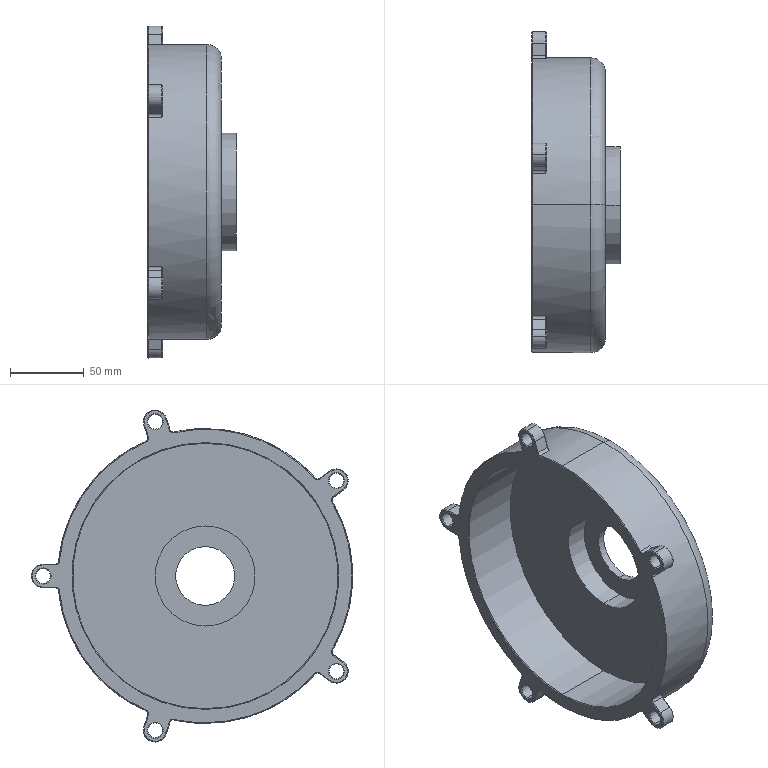Part | SolidWorks | 1 solid | 137 faces | box 60 x 218 x 225.232 mm | volume 538282 mm3 | cone 56 | plane 40 | cylinder 39 | torus 2 | commonest cylinder face diameters 4 x12 10 x10 16 x7 40 x2 68 x2 80 x2